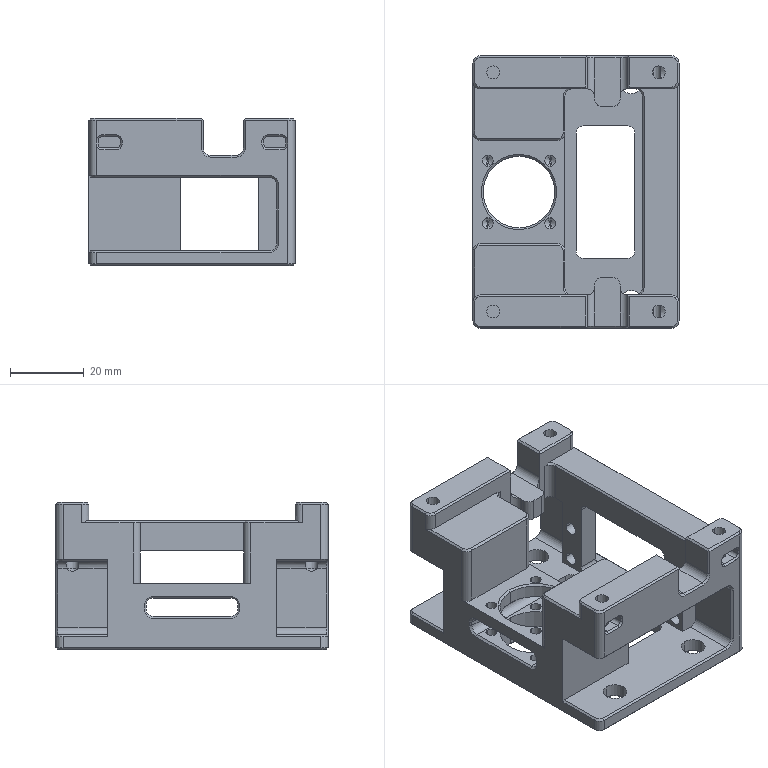NC program | Mastercam | posted with a generic post | part box 56 x 74 x 40 mm
Lines 4683 to 6480 of 45205, first 1525 of 1798 lines:
(3 FEM |TOOL - 3|DIA. OFF. - 3|LEN. - 3|TOOL DIA. - 3.)
N9410 T3 M6
N9412 G0 G54 G90 X10.5 Y9.5 C0. B0. S6000 M3
N9414 G43 H3 Z50.
N9416 Z1.
N9418 G1 Z0. F600.
N9420 X-10.5 Z-.111 F1500.
N9422 G3 X-11. Y9. Z-.116 J-.5
N9424 G1 Y8. Z-.121
N9426 X-10.976 Y7.845 Z-.122
N9428 X-10.905 Y7.706 Z-.123
N9430 X-10.794 Y7.595
N9432 X-10.655 Y7.524 Z-.124
N9434 X-10.5 Y7.5 Z-.125
N9436 X10.5 Z-.236
N9438 G3 X11. Y8. Z-.241 J.5
N9440 G1 Y9. Z-.246
N9442 X10.976 Y9.155 Z-.247
N9444 X10.905 Y9.294 Z-.248
N9446 X10.794 Y9.405
N9448 X10.655 Y9.476 Z-.249
N9450 X10.5 Y9.5 Z-.25
N9452 X-10.5 Z-.361
N9454 G3 X-11. Y9. Z-.366 J-.5
N9456 G1 Y8. Z-.371
N9458 X-10.976 Y7.845 Z-.372
N9460 X-10.905 Y7.706 Z-.373
N9462 X-10.794 Y7.595
N9464 X-10.655 Y7.524 Z-.374
N9466 X-10.5 Y7.5 Z-.375
N9468 X10.5 Z-.486
N9470 G3 X11. Y8. Z-.491 J.5
N9472 G1 Y9. Z-.496
N9474 X10.976 Y9.155 Z-.497
N9476 X10.905 Y9.294 Z-.498
N9478 X10.794 Y9.405
N9480 X10.655 Y9.476 Z-.499
N9482 X10.5 Y9.5 Z-.5
N9484 X-10.5 Z-.611
N9486 G3 X-11. Y9. Z-.616 J-.5
N9488 G1 Y8. Z-.621
N9490 X-10.976 Y7.845 Z-.622
N9492 X-10.905 Y7.706 Z-.623
N9494 X-10.794 Y7.595
N9496 X-10.655 Y7.524 Z-.624
N9498 X-10.5 Y7.5 Z-.625
N9500 X10.5 Z-.736
N9502 G3 X11. Y8. Z-.741 J.5
N9504 G1 Y9. Z-.746
N9506 X10.976 Y9.155 Z-.747
N9508 X10.905 Y9.294 Z-.748
N9510 X10.794 Y9.405
N9512 X10.655 Y9.476 Z-.749
N9514 X10.5 Y9.5 Z-.75
N9516 X-10.5 Z-.861
N9518 G3 X-11. Y9. Z-.866 J-.5
N9520 G1 Y8. Z-.871
N9522 X-10.976 Y7.845 Z-.872
N9524 X-10.905 Y7.706 Z-.873
N9526 X-10.794 Y7.595
N9528 X-10.655 Y7.524 Z-.874
N9530 X-10.5 Y7.5 Z-.875
N9532 X10.5 Z-.986
N9534 G3 X11. Y8. Z-.991 J.5
N9536 G1 Y9. Z-.996
N9538 X10.976 Y9.155 Z-.997
N9540 X10.905 Y9.294 Z-.998
N9542 X10.794 Y9.405
N9544 X10.655 Y9.476 Z-.999
N9546 X10.5 Y9.5 Z-1.
N9548 X-10.5 Z-1.111
N9550 G3 X-11. Y9. Z-1.116 J-.5
N9552 G1 Y8. Z-1.121
N9554 X-10.976 Y7.845 Z-1.122
N9556 X-10.905 Y7.706 Z-1.123
N9558 X-10.794 Y7.595
N9560 X-10.655 Y7.524 Z-1.124
N9562 X-10.5 Y7.5 Z-1.125
N9564 X10.5 Z-1.236
N9566 G3 X11. Y8. Z-1.241 J.5
N9568 G1 Y9. Z-1.246
N9570 X10.976 Y9.155 Z-1.247
N9572 X10.905 Y9.294 Z-1.248
N9574 X10.794 Y9.405
N9576 X10.655 Y9.476 Z-1.249
N9578 X10.5 Y9.5 Z-1.25
N9580 X-10.5 Z-1.361
N9582 G3 X-11. Y9. Z-1.366 J-.5
N9584 G1 Y8. Z-1.371
N9586 X-10.976 Y7.845 Z-1.372
N9588 X-10.905 Y7.706 Z-1.373
N9590 X-10.794 Y7.595
N9592 X-10.655 Y7.524 Z-1.374
N9594 X-10.5 Y7.5 Z-1.375
N9596 X10.5 Z-1.486
N9598 G3 X11. Y8. Z-1.491 J.5
N9600 G1 Y9. Z-1.496
N9602 X10.976 Y9.155 Z-1.497
N9604 X10.905 Y9.294 Z-1.498
N9606 X10.794 Y9.405
N9608 X10.655 Y9.476 Z-1.499
N9610 X10.5 Y9.5 Z-1.5
N9612 X-10.5 Z-1.611
N9614 G3 X-11. Y9. Z-1.616 J-.5
N9616 G1 Y8. Z-1.621
N9618 X-10.976 Y7.845 Z-1.622
N9620 X-10.905 Y7.706 Z-1.623
N9622 X-10.794 Y7.595
N9624 X-10.655 Y7.524 Z-1.624
N9626 X-10.5 Y7.5 Z-1.625
N9628 X10.5 Z-1.736
N9630 G3 X11. Y8. Z-1.741 J.5
N9632 G1 Y9. Z-1.746
N9634 X10.976 Y9.155 Z-1.747
N9636 X10.905 Y9.294 Z-1.748
N9638 X10.794 Y9.405
N9640 X10.655 Y9.476 Z-1.749
N9642 X10.5 Y9.5 Z-1.75
N9644 X-10.5 Z-1.861
N9646 G3 X-11. Y9. Z-1.866 J-.5
N9648 G1 Y8. Z-1.871
N9650 X-10.976 Y7.845 Z-1.872
N9652 X-10.905 Y7.706 Z-1.873
N9654 X-10.794 Y7.595
N9656 X-10.655 Y7.524 Z-1.874
N9658 X-10.5 Y7.5 Z-1.875
N9660 X10.5 Z-1.986
N9662 G3 X11. Y8. Z-1.991 J.5
N9664 G1 Y9. Z-1.996
N9666 X10.976 Y9.155 Z-1.997
N9668 X10.905 Y9.294 Z-1.998
N9670 X10.794 Y9.405
N9672 X10.655 Y9.476 Z-1.999
N9674 X10.5 Y9.5 Z-2.
N9676 X-10.5 Z-2.111
N9678 G3 X-11. Y9. Z-2.116 J-.5
N9680 G1 Y8. Z-2.121
N9682 X-10.976 Y7.845 Z-2.122
N9684 X-10.905 Y7.706 Z-2.123
N9686 X-10.794 Y7.595
N9688 X-10.655 Y7.524 Z-2.124
N9690 X-10.5 Y7.5 Z-2.125
N9692 X10.5 Z-2.236
N9694 G3 X11. Y8. Z-2.241 J.5
N9696 G1 Y9. Z-2.246
N9698 X10.976 Y9.155 Z-2.247
N9700 X10.905 Y9.294 Z-2.248
N9702 X10.794 Y9.405
N9704 X10.655 Y9.476 Z-2.249
N9706 X10.5 Y9.5 Z-2.25
N9708 X-10.5 Z-2.361
N9710 G3 X-11. Y9. Z-2.366 J-.5
N9712 G1 Y8. Z-2.371
N9714 X-10.976 Y7.845 Z-2.372
N9716 X-10.905 Y7.706 Z-2.373
N9718 X-10.794 Y7.595
N9720 X-10.655 Y7.524 Z-2.374
N9722 X-10.5 Y7.5 Z-2.375
N9724 X10.5 Z-2.486
N9726 G3 X11. Y8. Z-2.491 J.5
N9728 G1 Y9. Z-2.496
N9730 X10.976 Y9.155 Z-2.497
N9732 X10.905 Y9.294 Z-2.498
N9734 X10.794 Y9.405
N9736 X10.655 Y9.476 Z-2.499
N9738 X10.5 Y9.5 Z-2.5
N9740 X-10.5 Z-2.611
N9742 G3 X-11. Y9. Z-2.616 J-.5
N9744 G1 Y8. Z-2.621
N9746 X-10.976 Y7.845 Z-2.622
N9748 X-10.905 Y7.706 Z-2.623
N9750 X-10.794 Y7.595
N9752 X-10.655 Y7.524 Z-2.624
N9754 X-10.5 Y7.5 Z-2.625
N9756 X10.5 Z-2.736
N9758 G3 X11. Y8. Z-2.741 J.5
N9760 G1 Y9. Z-2.746
N9762 X10.976 Y9.155 Z-2.747
N9764 X10.905 Y9.294 Z-2.748
N9766 X10.794 Y9.405
N9768 X10.655 Y9.476 Z-2.749
N9770 X10.5 Y9.5 Z-2.75
N9772 X-10.5 Z-2.861
N9774 G3 X-11. Y9. Z-2.866 J-.5
N9776 G1 Y8. Z-2.871
N9778 X-10.976 Y7.845 Z-2.872
N9780 X-10.905 Y7.706 Z-2.873
N9782 X-10.794 Y7.595
N9784 X-10.655 Y7.524 Z-2.874
N9786 X-10.5 Y7.5 Z-2.875
N9788 X10.5 Z-2.986
N9790 G3 X11. Y8. Z-2.991 J.5
N9792 G1 Y9. Z-2.996
N9794 X10.976 Y9.155 Z-2.997
N9796 X10.905 Y9.294 Z-2.998
N9798 X10.794 Y9.405
N9800 X10.655 Y9.476 Z-2.999
N9802 X10.5 Y9.5 Z-3.
N9804 X-10.5 Z-3.111
N9806 G3 X-11. Y9. Z-3.116 J-.5
N9808 G1 Y8. Z-3.121
N9810 X-10.976 Y7.845 Z-3.122
N9812 X-10.905 Y7.706 Z-3.123
N9814 X-10.794 Y7.595
N9816 X-10.655 Y7.524 Z-3.124
N9818 X-10.5 Y7.5 Z-3.125
N9820 X10.5 Z-3.236
N9822 G3 X11. Y8. Z-3.241 J.5
N9824 G1 Y9. Z-3.246
N9826 X10.976 Y9.155 Z-3.247
N9828 X10.905 Y9.294 Z-3.248
N9830 X10.794 Y9.405
N9832 X10.655 Y9.476 Z-3.249
N9834 X10.5 Y9.5 Z-3.25
N9836 X-10.5 Z-3.361
N9838 G3 X-11. Y9. Z-3.366 J-.5
N9840 G1 Y8. Z-3.371
N9842 X-10.976 Y7.845 Z-3.372
N9844 X-10.905 Y7.706 Z-3.373
N9846 X-10.794 Y7.595
N9848 X-10.655 Y7.524 Z-3.374
N9850 X-10.5 Y7.5 Z-3.375
N9852 X10.5 Z-3.486
N9854 G3 X11. Y8. Z-3.491 J.5
N9856 G1 Y9. Z-3.496
N9858 X10.976 Y9.155 Z-3.497
N9860 X10.905 Y9.294 Z-3.498
N9862 X10.794 Y9.405
N9864 X10.655 Y9.476 Z-3.499
N9866 X10.5 Y9.5 Z-3.5
N9868 X-10.5 Z-3.611
N9870 G3 X-11. Y9. Z-3.616 J-.5
N9872 G1 Y8. Z-3.621
N9874 X-10.976 Y7.845 Z-3.622
N9876 X-10.905 Y7.706 Z-3.623
N9878 X-10.794 Y7.595
N9880 X-10.655 Y7.524 Z-3.624
N9882 X-10.5 Y7.5 Z-3.625
N9884 X10.5 Z-3.736
N9886 G3 X11. Y8. Z-3.741 J.5
N9888 G1 Y9. Z-3.746
N9890 X10.976 Y9.155 Z-3.747
N9892 X10.905 Y9.294 Z-3.748
N9894 X10.794 Y9.405
N9896 X10.655 Y9.476 Z-3.749
N9898 X10.5 Y9.5 Z-3.75
N9900 X-10.5 Z-3.861
N9902 G3 X-11. Y9. Z-3.866 J-.5
N9904 G1 Y8. Z-3.871
N9906 X-10.976 Y7.845 Z-3.872
N9908 X-10.905 Y7.706 Z-3.873
N9910 X-10.794 Y7.595
N9912 X-10.655 Y7.524 Z-3.874
N9914 X-10.5 Y7.5 Z-3.875
N9916 X10.5 Z-3.986
N9918 G3 X11. Y8. Z-3.991 J.5
N9920 G1 Y9. Z-3.996
N9922 X10.976 Y9.155 Z-3.997
N9924 X10.905 Y9.294 Z-3.998
N9926 X10.794 Y9.405
N9928 X10.655 Y9.476 Z-3.999
N9930 X10.5 Y9.5 Z-4.
N9932 X-10.5 Z-4.111
N9934 G3 X-11. Y9. Z-4.116 J-.5
N9936 G1 Y8. Z-4.121
N9938 X-10.976 Y7.845 Z-4.122
N9940 X-10.905 Y7.706 Z-4.123
N9942 X-10.794 Y7.595
N9944 X-10.655 Y7.524 Z-4.124
N9946 X-10.5 Y7.5 Z-4.125
N9948 X10.5 Z-4.236
N9950 G3 X11. Y8. Z-4.241 J.5
N9952 G1 Y9. Z-4.246
N9954 X10.976 Y9.155 Z-4.247
N9956 X10.905 Y9.294 Z-4.248
N9958 X10.794 Y9.405
N9960 X10.655 Y9.476 Z-4.249
N9962 X10.5 Y9.5 Z-4.25
N9964 X-10.5 Z-4.361
N9966 G3 X-11. Y9. Z-4.366 J-.5
N9968 G1 Y8. Z-4.371
N9970 X-10.976 Y7.845 Z-4.372
N9972 X-10.905 Y7.706 Z-4.373
N9974 X-10.794 Y7.595
N9976 X-10.655 Y7.524 Z-4.374
N9978 X-10.5 Y7.5 Z-4.375
N9980 X10.5 Z-4.486
N9982 G3 X11. Y8. Z-4.491 J.5
N9984 G1 Y9. Z-4.496
N9986 X10.976 Y9.155 Z-4.497
N9988 X10.905 Y9.294 Z-4.498
N9990 X10.794 Y9.405
N9992 X10.655 Y9.476 Z-4.499
N9994 X10.5 Y9.5 Z-4.5
N9996 X-10.5 Z-4.611
N9998 G3 X-11. Y9. Z-4.616 J-.5
N100 G1 Y8. Z-4.621
N102 X-10.976 Y7.845 Z-4.622
N104 X-10.905 Y7.706 Z-4.623
N106 X-10.794 Y7.595
N108 X-10.655 Y7.524 Z-4.624
N110 X-10.5 Y7.5 Z-4.625
N112 X10.5 Z-4.736
N114 G3 X11. Y8. Z-4.741 J.5
N116 G1 Y9. Z-4.746
N118 X10.976 Y9.155 Z-4.747
N120 X10.905 Y9.294 Z-4.748
N122 X10.794 Y9.405
N124 X10.655 Y9.476 Z-4.749
N126 X10.5 Y9.5 Z-4.75
N128 X-10.5 Z-4.861
N130 G3 X-11. Y9. Z-4.866 J-.5
N132 G1 Y8. Z-4.871
N134 X-10.976 Y7.845 Z-4.872
N136 X-10.905 Y7.706 Z-4.873
N138 X-10.794 Y7.595
N140 X-10.655 Y7.524 Z-4.874
N142 X-10.5 Y7.5 Z-4.875
N144 X10.5 Z-4.986
N146 G3 X11. Y8. Z-4.991 J.5
N148 G1 Y9. Z-4.996
N150 X10.976 Y9.155 Z-4.997
N152 X10.905 Y9.294 Z-4.998
N154 X10.794 Y9.405
N156 X10.655 Y9.476 Z-4.999
N158 X10.5 Y9.5 Z-5.
N160 X-10.5 Z-5.111
N162 G3 X-11. Y9. Z-5.116 J-.5
N164 G1 Y8. Z-5.121
N166 X-10.976 Y7.845 Z-5.122
N168 X-10.905 Y7.706 Z-5.123
N170 X-10.794 Y7.595
N172 X-10.655 Y7.524 Z-5.124
N174 X-10.5 Y7.5 Z-5.125
N176 X10.5 Z-5.236
N178 G3 X11. Y8. Z-5.241 J.5
N180 G1 Y9. Z-5.246
N182 X10.976 Y9.155 Z-5.247
N184 X10.905 Y9.294 Z-5.248
N186 X10.794 Y9.405
N188 X10.655 Y9.476 Z-5.249
N190 X10.5 Y9.5 Z-5.25
N192 X-10.5 Z-5.361
N194 G3 X-11. Y9. Z-5.366 J-.5
N196 G1 Y8. Z-5.371
N198 X-10.976 Y7.845 Z-5.372
N200 X-10.905 Y7.706 Z-5.373
N202 X-10.794 Y7.595
N204 X-10.655 Y7.524 Z-5.374
N206 X-10.5 Y7.5 Z-5.375
N208 X10.5 Z-5.486
N210 G3 X11. Y8. Z-5.491 J.5
N212 G1 Y9. Z-5.496
N214 X10.976 Y9.155 Z-5.497
N216 X10.905 Y9.294 Z-5.498
N218 X10.794 Y9.405
N220 X10.655 Y9.476 Z-5.499
N222 X10.5 Y9.5 Z-5.5
N224 X-10.5 Z-5.611
N226 G3 X-11. Y9. Z-5.616 J-.5
N228 G1 Y8. Z-5.621
N230 X-10.976 Y7.845 Z-5.622
N232 X-10.905 Y7.706 Z-5.623
N234 X-10.794 Y7.595
N236 X-10.655 Y7.524 Z-5.624
N238 X-10.5 Y7.5 Z-5.625
N240 X10.5 Z-5.736
N242 G3 X11. Y8. Z-5.741 J.5
N244 G1 Y9. Z-5.746
N246 X10.976 Y9.155 Z-5.747
N248 X10.905 Y9.294 Z-5.748
N250 X10.794 Y9.405
N252 X10.655 Y9.476 Z-5.749
N254 X10.5 Y9.5 Z-5.75
N256 X-10.5 Z-5.861
N258 G3 X-11. Y9. Z-5.866 J-.5
N260 G1 Y8. Z-5.871
N262 X-10.976 Y7.845 Z-5.872
N264 X-10.905 Y7.706 Z-5.873
N266 X-10.794 Y7.595
N268 X-10.655 Y7.524 Z-5.874
N270 X-10.5 Y7.5 Z-5.875
N272 X10.5 Z-5.986
N274 G3 X11. Y8. Z-5.991 J.5
N276 G1 Y9. Z-5.996
N278 X10.976 Y9.155 Z-5.997
N280 X10.905 Y9.294 Z-5.998
N282 X10.794 Y9.405
N284 X10.655 Y9.476 Z-5.999
N286 X10.5 Y9.5 Z-6.
N288 X-10.5 Z-6.111
N290 G3 X-11. Y9. Z-6.116 J-.5
N292 G1 Y8. Z-6.121
N294 X-10.976 Y7.845 Z-6.122
N296 X-10.905 Y7.706 Z-6.123
N298 X-10.794 Y7.595
N300 X-10.655 Y7.524 Z-6.124
N302 X-10.5 Y7.5 Z-6.125
N304 X10.5 Z-6.236
N306 G3 X11. Y8. Z-6.241 J.5
N308 G1 Y9. Z-6.246
N310 X10.976 Y9.155 Z-6.247
N312 X10.905 Y9.294 Z-6.248
N314 X10.794 Y9.405
N316 X10.655 Y9.476 Z-6.249
N318 X10.5 Y9.5 Z-6.25
N320 X-10.5 Z-6.361
N322 G3 X-11. Y9. Z-6.366 J-.5
N324 G1 Y8. Z-6.371
N326 X-10.976 Y7.845 Z-6.372
N328 X-10.905 Y7.706 Z-6.373
N330 X-10.794 Y7.595
N332 X-10.655 Y7.524 Z-6.374
N334 X-10.5 Y7.5 Z-6.375
N336 X10.5 Z-6.486
N338 G3 X11. Y8. Z-6.491 J.5
N340 G1 Y9. Z-6.496
N342 X10.976 Y9.155 Z-6.497
N344 X10.905 Y9.294 Z-6.498
N346 X10.794 Y9.405
N348 X10.655 Y9.476 Z-6.499
N350 X10.5 Y9.5 Z-6.5
N352 X-10.5 Z-6.611
N354 G3 X-11. Y9. Z-6.616 J-.5
N356 G1 Y8. Z-6.621
N358 X-10.976 Y7.845 Z-6.622
N360 X-10.905 Y7.706 Z-6.623
N362 X-10.794 Y7.595
N364 X-10.655 Y7.524 Z-6.624
N366 X-10.5 Y7.5 Z-6.625
N368 X10.5 Z-6.736
N370 G3 X11. Y8. Z-6.741 J.5
N372 G1 Y9. Z-6.746
N374 X10.976 Y9.155 Z-6.747
N376 X10.905 Y9.294 Z-6.748
N378 X10.794 Y9.405
N380 X10.655 Y9.476 Z-6.749
N382 X10.5 Y9.5 Z-6.75
N384 X-10.5 Z-6.861
N386 G3 X-11. Y9. Z-6.866 J-.5
N388 G1 Y8. Z-6.871
N390 X-10.976 Y7.845 Z-6.872
N392 X-10.905 Y7.706 Z-6.873
N394 X-10.794 Y7.595
N396 X-10.655 Y7.524 Z-6.874
N398 X-10.5 Y7.5 Z-6.875
N400 X10.5 Z-6.986
N402 G3 X11. Y8. Z-6.991 J.5
N404 G1 Y9. Z-6.996
N406 X10.976 Y9.155 Z-6.997
N408 X10.905 Y9.294 Z-6.998
N410 X10.794 Y9.405
N412 X10.655 Y9.476 Z-6.999
N414 X10.5 Y9.5 Z-7.
N416 X-10.5 Z-7.111
N418 G3 X-11. Y9. Z-7.116 J-.5
N420 G1 Y8. Z-7.121
N422 X-10.976 Y7.845 Z-7.122
N424 X-10.905 Y7.706 Z-7.123
N426 X-10.794 Y7.595
N428 X-10.655 Y7.524 Z-7.124
N430 X-10.5 Y7.5 Z-7.125
N432 X10.5 Z-7.236
N434 G3 X11. Y8. Z-7.241 J.5
N436 G1 Y9. Z-7.246
N438 X10.976 Y9.155 Z-7.247
N440 X10.905 Y9.294 Z-7.248
N442 X10.794 Y9.405
N444 X10.655 Y9.476 Z-7.249
N446 X10.5 Y9.5 Z-7.25
N448 X-10.5 Z-7.361
N450 G3 X-11. Y9. Z-7.366 J-.5
N452 G1 Y8. Z-7.371
N454 X-10.976 Y7.845 Z-7.372
N456 X-10.905 Y7.706 Z-7.373
N458 X-10.794 Y7.595
N460 X-10.655 Y7.524 Z-7.374
N462 X-10.5 Y7.5 Z-7.375
N464 X10.5 Z-7.486
N466 G3 X11. Y8. Z-7.491 J.5
N468 G1 Y9. Z-7.496
N470 X10.976 Y9.155 Z-7.497
N472 X10.905 Y9.294 Z-7.498
N474 X10.794 Y9.405
N476 X10.655 Y9.476 Z-7.499
N478 X10.5 Y9.5 Z-7.5
N480 X-10.5 Z-7.611
N482 G3 X-11. Y9. Z-7.616 J-.5
N484 G1 Y8. Z-7.621
N486 X-10.976 Y7.845 Z-7.622
N488 X-10.905 Y7.706 Z-7.623
N490 X-10.794 Y7.595
N492 X-10.655 Y7.524 Z-7.624
N494 X-10.5 Y7.5 Z-7.625
N496 X10.5 Z-7.736
N498 G3 X11. Y8. Z-7.741 J.5
N500 G1 Y9. Z-7.746
N502 X10.976 Y9.155 Z-7.747
N504 X10.905 Y9.294 Z-7.748
N506 X10.794 Y9.405
N508 X10.655 Y9.476 Z-7.749
N510 X10.5 Y9.5 Z-7.75
N512 X-10.5 Z-7.861
N514 G3 X-11. Y9. Z-7.866 J-.5
N516 G1 Y8. Z-7.871
N518 X-10.976 Y7.845 Z-7.872
N520 X-10.905 Y7.706 Z-7.873
N522 X-10.794 Y7.595
N524 X-10.655 Y7.524 Z-7.874
N526 X-10.5 Y7.5 Z-7.875
N528 X10.5 Z-7.986
N530 G3 X11. Y8. Z-7.991 J.5
N532 G1 Y9. Z-7.996
N534 X10.976 Y9.155 Z-7.997
N536 X10.905 Y9.294 Z-7.998
N538 X10.794 Y9.405
N540 X10.655 Y9.476 Z-7.999
N542 X10.5 Y9.5 Z-8.
N544 X-10.5 Z-8.111
N546 G3 X-11. Y9. Z-8.116 J-.5
N548 G1 Y8. Z-8.121
N550 X-10.976 Y7.845 Z-8.122
N552 X-10.905 Y7.706 Z-8.123
N554 X-10.794 Y7.595
N556 X-10.655 Y7.524 Z-8.124
N558 X-10.5 Y7.5 Z-8.125
N560 X10.5 Z-8.236
N562 G3 X11. Y8. Z-8.241 J.5
N564 G1 Y9. Z-8.246
N566 X10.976 Y9.155 Z-8.247
N568 X10.905 Y9.294 Z-8.248
N570 X10.794 Y9.405
N572 X10.655 Y9.476 Z-8.249
N574 X10.5 Y9.5 Z-8.25
N576 X-10.5 Z-8.361
N578 G3 X-11. Y9. Z-8.366 J-.5
N580 G1 Y8. Z-8.371
N582 X-10.976 Y7.845 Z-8.372
N584 X-10.905 Y7.706 Z-8.373
N586 X-10.794 Y7.595
N588 X-10.655 Y7.524 Z-8.374
N590 X-10.5 Y7.5 Z-8.375
N592 X10.5 Z-8.486
N594 G3 X11. Y8. Z-8.491 J.5
N596 G1 Y9. Z-8.496
N598 X10.976 Y9.155 Z-8.497
N600 X10.905 Y9.294 Z-8.498
N602 X10.794 Y9.405
N604 X10.655 Y9.476 Z-8.499
N606 X10.5 Y9.5 Z-8.5
N608 X-10.5 Z-8.611
N610 G3 X-11. Y9. Z-8.616 J-.5
N612 G1 Y8. Z-8.621
N614 X-10.976 Y7.845 Z-8.622
N616 X-10.905 Y7.706 Z-8.623
N618 X-10.794 Y7.595
N620 X-10.655 Y7.524 Z-8.624
N622 X-10.5 Y7.5 Z-8.625
N624 X10.5 Z-8.736
N626 G3 X11. Y8. Z-8.741 J.5
N628 G1 Y9. Z-8.746
N630 X10.976 Y9.155 Z-8.747
N632 X10.905 Y9.294 Z-8.748
N634 X10.794 Y9.405
N636 X10.655 Y9.476 Z-8.749
N638 X10.5 Y9.5 Z-8.75
N640 X-10.5 Z-8.861
N642 G3 X-11. Y9. Z-8.866 J-.5
N644 G1 Y8. Z-8.871
N646 X-10.976 Y7.845 Z-8.872
N648 X-10.905 Y7.706 Z-8.873
N650 X-10.794 Y7.595
N652 X-10.655 Y7.524 Z-8.874
N654 X-10.5 Y7.5 Z-8.875
N656 X10.5 Z-8.986
N658 G3 X11. Y8. Z-8.991 J.5
N660 G1 Y9. Z-8.996
N662 X10.976 Y9.155 Z-8.997
N664 X10.905 Y9.294 Z-8.998
N666 X10.794 Y9.405
N668 X10.655 Y9.476 Z-8.999
N670 X10.5 Y9.5 Z-9.
N672 X-10.5 Z-9.111
N674 G3 X-11. Y9. Z-9.116 J-.5
N676 G1 Y8. Z-9.121
N678 X-10.976 Y7.845 Z-9.122
N680 X-10.905 Y7.706 Z-9.123
N682 X-10.794 Y7.595
N684 X-10.655 Y7.524 Z-9.124
N686 X-10.5 Y7.5 Z-9.125
N688 X10.5 Z-9.236
N690 G3 X11. Y8. Z-9.241 J.5
N692 G1 Y9. Z-9.246
N694 X10.976 Y9.155 Z-9.247
N696 X10.905 Y9.294 Z-9.248
N698 X10.794 Y9.405
N700 X10.655 Y9.476 Z-9.249
N702 X10.5 Y9.5 Z-9.25
N704 X-10.5 Z-9.361
N706 G3 X-11. Y9. Z-9.366 J-.5
N708 G1 Y8. Z-9.371
N710 X-10.976 Y7.845 Z-9.372
N712 X-10.905 Y7.706 Z-9.373
N714 X-10.794 Y7.595
N716 X-10.655 Y7.524 Z-9.374
N718 X-10.5 Y7.5 Z-9.375
N720 X10.5 Z-9.486
N722 G3 X11. Y8. Z-9.491 J.5
N724 G1 Y9. Z-9.496
N726 X10.976 Y9.155 Z-9.497
N728 X10.905 Y9.294 Z-9.498
N730 X10.794 Y9.405
N732 X10.655 Y9.476 Z-9.499
N734 X10.5 Y9.5 Z-9.5
N736 X-10.5 Z-9.611
N738 G3 X-11. Y9. Z-9.616 J-.5
N740 G1 Y8. Z-9.621
N742 X-10.976 Y7.845 Z-9.622
N744 X-10.905 Y7.706 Z-9.623
N746 X-10.794 Y7.595
N748 X-10.655 Y7.524 Z-9.624
N750 X-10.5 Y7.5 Z-9.625
N752 X10.5 Z-9.736
N754 G3 X11. Y8. Z-9.741 J.5
N756 G1 Y9. Z-9.746
N758 X10.976 Y9.155 Z-9.747
N760 X10.905 Y9.294 Z-9.748
N762 X10.794 Y9.405
N764 X10.655 Y9.476 Z-9.749
N766 X10.5 Y9.5 Z-9.75
N768 X-10.5 Z-9.861
N770 G3 X-11. Y9. Z-9.866 J-.5
N772 G1 Y8. Z-9.871
N774 X-10.976 Y7.845 Z-9.872
N776 X-10.905 Y7.706 Z-9.873
N778 X-10.794 Y7.595
N780 X-10.655 Y7.524 Z-9.874
N782 X-10.5 Y7.5 Z-9.875
N784 X10.5 Z-9.986
N786 G3 X11. Y8. Z-9.991 J.5
N788 G1 Y9. Z-9.996
N790 X10.976 Y9.155 Z-9.997
N792 X10.905 Y9.294 Z-9.998
N794 X10.794 Y9.405
N796 X10.655 Y9.476 Z-9.999
N798 X10.5 Y9.5 Z-10.
N800 X-10.5 Z-10.111
N802 G3 X-11. Y9. Z-10.116 J-.5
N804 G1 Y8. Z-10.121
N806 X-10.976 Y7.845 Z-10.122
N808 X-10.905 Y7.706 Z-10.123
N810 X-10.794 Y7.595
N812 X-10.655 Y7.524 Z-10.124
N814 X-10.5 Y7.5 Z-10.125
N816 X10.5 Z-10.236
N818 G3 X11. Y8. Z-10.241 J.5
N820 G1 Y9. Z-10.246
N822 X10.976 Y9.155 Z-10.247
N824 X10.905 Y9.294 Z-10.248
N826 X10.794 Y9.405
N828 X10.655 Y9.476 Z-10.249
N830 X10.5 Y9.5 Z-10.25
N832 X-10.5 Z-10.361
N834 G3 X-11. Y9. Z-10.366 J-.5
N836 G1 Y8. Z-10.371
N838 X-10.976 Y7.845 Z-10.372
N840 X-10.905 Y7.706 Z-10.373
N842 X-10.794 Y7.595
N844 X-10.655 Y7.524 Z-10.374
N846 X-10.5 Y7.5 Z-10.375
N848 X10.5 Z-10.486
N850 G3 X11. Y8. Z-10.491 J.5
N852 G1 Y9. Z-10.496
N854 X10.976 Y9.155 Z-10.497
N856 X10.905 Y9.294 Z-10.498
N858 X10.794 Y9.405
N860 X10.655 Y9.476 Z-10.499
N862 X10.5 Y9.5 Z-10.5
N864 X-10.5 Z-10.611
N866 G3 X-11. Y9. Z-10.616 J-.5
N868 G1 Y8. Z-10.621
N870 X-10.976 Y7.845 Z-10.622
N872 X-10.905 Y7.706 Z-10.623
N874 X-10.794 Y7.595
N876 X-10.655 Y7.524 Z-10.624
N878 X-10.5 Y7.5 Z-10.625
N880 X10.5 Z-10.736
N882 G3 X11. Y8. Z-10.741 J.5
N884 G1 Y9. Z-10.746
N886 X10.976 Y9.155 Z-10.747
N888 X10.905 Y9.294 Z-10.748
N890 X10.794 Y9.405
N892 X10.655 Y9.476 Z-10.749
N894 X10.5 Y9.5 Z-10.75
N896 X-10.5 Z-10.861
N898 G3 X-11. Y9. Z-10.866 J-.5
N900 G1 Y8. Z-10.871
N902 X-10.976 Y7.845 Z-10.872
N904 X-10.905 Y7.706 Z-10.873
N906 X-10.794 Y7.595
N908 X-10.655 Y7.524 Z-10.874
N910 X-10.5 Y7.5 Z-10.875
N912 X10.5 Z-10.986
N914 G3 X11. Y8. Z-10.991 J.5
N916 G1 Y9. Z-10.996
N918 X10.976 Y9.155 Z-10.997
N920 X10.905 Y9.294 Z-10.998
N922 X10.794 Y9.405
N924 X10.655 Y9.476 Z-10.999
N926 X10.5 Y9.5 Z-11.
N928 X-10.5 Z-11.111
N930 G3 X-11. Y9. Z-11.116 J-.5
N932 G1 Y8. Z-11.121
N934 X-10.976 Y7.845 Z-11.122
N936 X-10.905 Y7.706 Z-11.123
N938 X-10.794 Y7.595
N940 X-10.655 Y7.524 Z-11.124
N942 X-10.5 Y7.5 Z-11.125
N944 X10.5 Z-11.236
N946 G3 X11. Y8. Z-11.241 J.5
N948 G1 Y9. Z-11.246
N950 X10.976 Y9.155 Z-11.247
N952 X10.905 Y9.294 Z-11.248
N954 X10.794 Y9.405
N956 X10.655 Y9.476 Z-11.249
N958 X10.5 Y9.5 Z-11.25
N960 X-10.5 Z-11.361
N962 G3 X-11. Y9. Z-11.366 J-.5
N964 G1 Y8. Z-11.371
N966 X-10.976 Y7.845 Z-11.372
N968 X-10.905 Y7.706 Z-11.373
N970 X-10.794 Y7.595
N972 X-10.655 Y7.524 Z-11.374
N974 X-10.5 Y7.5 Z-11.375
N976 X10.5 Z-11.486
N978 G3 X11. Y8. Z-11.491 J.5
N980 G1 Y9. Z-11.496
N982 X10.976 Y9.155 Z-11.497
N984 X10.905 Y9.294 Z-11.498
N986 X10.794 Y9.405
N988 X10.655 Y9.476 Z-11.499
N990 X10.5 Y9.5 Z-11.5
N992 X-10.5 Z-11.611
N994 G3 X-11. Y9. Z-11.616 J-.5
N996 G1 Y8. Z-11.621
N998 X-10.976 Y7.845 Z-11.622
N1000 X-10.905 Y7.706 Z-11.623
N1002 X-10.794 Y7.595
N1004 X-10.655 Y7.524 Z-11.624
N1006 X-10.5 Y7.5 Z-11.625
N1008 X10.5 Z-11.736
N1010 G3 X11. Y8. Z-11.741 J.5
N1012 G1 Y9. Z-11.746
N1014 X10.976 Y9.155 Z-11.747
N1016 X10.905 Y9.294 Z-11.748
N1018 X10.794 Y9.405
N1020 X10.655 Y9.476 Z-11.749
N1022 X10.5 Y9.5 Z-11.75
N1024 X-10.5 Z-11.861
N1026 G3 X-11. Y9. Z-11.866 J-.5
N1028 G1 Y8. Z-11.871
N1030 X-10.976 Y7.845 Z-11.872
N1032 X-10.905 Y7.706 Z-11.873
N1034 X-10.794 Y7.595
N1036 X-10.655 Y7.524 Z-11.874
N1038 X-10.5 Y7.5 Z-11.875
N1040 X10.5 Z-11.986
N1042 G3 X11. Y8. Z-11.991 J.5
N1044 G1 Y9. Z-11.996
N1046 X10.976 Y9.155 Z-11.997
N1048 X10.905 Y9.294 Z-11.998
N1050 X10.794 Y9.405
N1052 X10.655 Y9.476 Z-11.999
N1054 X10.5 Y9.5 Z-12.
N1056 X-10.5 Z-12.111
N1058 G3 X-11. Y9. Z-12.116 J-.5
N1060 G1 Y8. Z-12.121
N1062 X-10.976 Y7.845 Z-12.122
N1064 X-10.905 Y7.706 Z-12.123
N1066 X-10.794 Y7.595
N1068 X-10.655 Y7.524 Z-12.124
N1070 X-10.5 Y7.5 Z-12.125
N1072 X10.5 Z-12.236
N1074 G3 X11. Y8. Z-12.241 J.5
N1076 G1 Y9. Z-12.246
N1078 X10.976 Y9.155 Z-12.247
N1080 X10.905 Y9.294 Z-12.248
N1082 X10.794 Y9.405
N1084 X10.655 Y9.476 Z-12.249
N1086 X10.5 Y9.5 Z-12.25
N1088 X-10.5 Z-12.361
N1090 G3 X-11. Y9. Z-12.366 J-.5
N1092 G1 Y8. Z-12.371
N1094 X-10.976 Y7.845 Z-12.372
N1096 X-10.905 Y7.706 Z-12.373
N1098 X-10.794 Y7.595
N1100 X-10.655 Y7.524 Z-12.374
N1102 X-10.5 Y7.5 Z-12.375
N1104 X10.5 Z-12.486
N1106 G3 X11. Y8. Z-12.491 J.5
N1108 G1 Y9. Z-12.496
N1110 X10.976 Y9.155 Z-12.497
N1112 X10.905 Y9.294 Z-12.498
N1114 X10.794 Y9.405
N1116 X10.655 Y9.476 Z-12.499
N1118 X10.5 Y9.5 Z-12.5
N1120 X-10.5 Z-12.611
N1122 G3 X-11. Y9. Z-12.616 J-.5
N1124 G1 Y8. Z-12.621
N1126 X-10.976 Y7.845 Z-12.622
N1128 X-10.905 Y7.706 Z-12.623
N1130 X-10.794 Y7.595
N1132 X-10.655 Y7.524 Z-12.624
N1134 X-10.5 Y7.5 Z-12.625
N1136 X10.5 Z-12.736
N1138 G3 X11. Y8. Z-12.741 J.5
N1140 G1 Y9. Z-12.746
N1142 X10.976 Y9.155 Z-12.747
N1144 X10.905 Y9.294 Z-12.748
N1146 X10.794 Y9.405
N1148 X10.655 Y9.476 Z-12.749
N1150 X10.5 Y9.5 Z-12.75
N1152 X-10.5 Z-12.861
N1154 G3 X-11. Y9. Z-12.866 J-.5
N1156 G1 Y8. Z-12.871
N1158 X-10.976 Y7.845 Z-12.872
N1160 X-10.905 Y7.706 Z-12.873
N1162 X-10.794 Y7.595
N1164 X-10.655 Y7.524 Z-12.874
N1166 X-10.5 Y7.5 Z-12.875
N1168 X10.5 Z-12.986
N1170 G3 X11. Y8. Z-12.991 J.5
N1172 G1 Y9. Z-12.996
N1174 X10.976 Y9.155 Z-12.997
N1176 X10.905 Y9.294 Z-12.998
N1178 X10.794 Y9.405
N1180 X10.655 Y9.476 Z-12.999
N1182 X10.5 Y9.5 Z-13.
N1184 X-10.5 Z-13.111
N1186 G3 X-11. Y9. Z-13.116 J-.5
N1188 G1 Y8. Z-13.121
N1190 X-10.976 Y7.845 Z-13.122
N1192 X-10.905 Y7.706 Z-13.123
N1194 X-10.794 Y7.595
N1196 X-10.655 Y7.524 Z-13.124
N1198 X-10.5 Y7.5 Z-13.125
N1200 X10.5 Z-13.236
N1202 G3 X11. Y8. Z-13.241 J.5
N1204 G1 Y9. Z-13.246
N1206 X10.976 Y9.155 Z-13.247
N1208 X10.905 Y9.294 Z-13.248
N1210 X10.794 Y9.405
N1212 X10.655 Y9.476 Z-13.249
N1214 X10.5 Y9.5 Z-13.25
N1216 X-10.5 Z-13.361
N1218 G3 X-11. Y9. Z-13.366 J-.5
N1220 G1 Y8. Z-13.371
N1222 X-10.976 Y7.845 Z-13.372
N1224 X-10.905 Y7.706 Z-13.373
N1226 X-10.794 Y7.595
N1228 X-10.655 Y7.524 Z-13.374
N1230 X-10.5 Y7.5 Z-13.375
N1232 X10.5 Z-13.486
N1234 G3 X11. Y8. Z-13.491 J.5
N1236 G1 Y9. Z-13.496
N1238 X10.976 Y9.155 Z-13.497
N1240 X10.905 Y9.294 Z-13.498
N1242 X10.794 Y9.405
N1244 X10.655 Y9.476 Z-13.499
N1246 X10.5 Y9.5 Z-13.5
N1248 X-10.5 Z-13.611
N1250 G3 X-11. Y9. Z-13.616 J-.5
N1252 G1 Y8. Z-13.621
N1254 X-10.976 Y7.845 Z-13.622
N1256 X-10.905 Y7.706 Z-13.623
N1258 X-10.794 Y7.595
N1260 X-10.655 Y7.524 Z-13.624
N1262 X-10.5 Y7.5 Z-13.625
N1264 X10.5 Z-13.736
N1266 G3 X11. Y8. Z-13.741 J.5
N1268 G1 Y9. Z-13.746
N1270 X10.976 Y9.155 Z-13.747
N1272 X10.905 Y9.294 Z-13.748
N1274 X10.794 Y9.405
N1276 X10.655 Y9.476 Z-13.749
N1278 X10.5 Y9.5 Z-13.75
N1280 X-10.5 Z-13.861
N1282 G3 X-11. Y9. Z-13.866 J-.5
N1284 G1 Y8. Z-13.871
N1286 X-10.976 Y7.845 Z-13.872
N1288 X-10.905 Y7.706 Z-13.873
N1290 X-10.794 Y7.595
N1292 X-10.655 Y7.524 Z-13.874
N1294 X-10.5 Y7.5 Z-13.875
N1296 X10.5 Z-13.986
N1298 G3 X11. Y8. Z-13.991 J.5
N1300 G1 Y9. Z-13.996
N1302 X10.976 Y9.155 Z-13.997
N1304 X10.905 Y9.294 Z-13.998
N1306 X10.794 Y9.405
N1308 X10.655 Y9.476 Z-13.999
N1310 X10.5 Y9.5 Z-14.
N1312 X-10.5 Z-14.111
N1314 G3 X-11. Y9. Z-14.116 J-.5
N1316 G1 Y8. Z-14.121
N1318 X-10.976 Y7.845 Z-14.122
N1320 X-10.905 Y7.706 Z-14.123
N1322 X-10.794 Y7.595
N1324 X-10.655 Y7.524 Z-14.124
N1326 X-10.5 Y7.5 Z-14.125
N1328 X10.5 Z-14.236
N1330 G3 X11. Y8. Z-14.241 J.5
N1332 G1 Y9. Z-14.246
N1334 X10.976 Y9.155 Z-14.247
N1336 X10.905 Y9.294 Z-14.248
N1338 X10.794 Y9.405
N1340 X10.655 Y9.476 Z-14.249
N1342 X10.5 Y9.5 Z-14.25
N1344 X-10.5 Z-14.361
N1346 G3 X-11. Y9. Z-14.366 J-.5
N1348 G1 Y8. Z-14.371
N1350 X-10.976 Y7.845 Z-14.372
N1352 X-10.905 Y7.706 Z-14.373
N1354 X-10.794 Y7.595
N1356 X-10.655 Y7.524 Z-14.374
N1358 X-10.5 Y7.5 Z-14.375
N1360 X10.5 Z-14.486
N1362 G3 X11. Y8. Z-14.491 J.5
N1364 G1 Y9. Z-14.496
N1366 X10.976 Y9.155 Z-14.497
N1368 X10.905 Y9.294 Z-14.498
N1370 X10.794 Y9.405
N1372 X10.655 Y9.476 Z-14.499
N1374 X10.5 Y9.5 Z-14.5
N1376 X-10.5 Z-14.611
N1378 G3 X-11. Y9. Z-14.616 J-.5
N1380 G1 Y8. Z-14.621
N1382 X-10.976 Y7.845 Z-14.622
N1384 X-10.905 Y7.706 Z-14.623
N1386 X-10.794 Y7.595
N1388 X-10.655 Y7.524 Z-14.624
N1390 X-10.5 Y7.5 Z-14.625
N1392 X10.5 Z-14.736
N1394 G3 X11. Y8. Z-14.741 J.5
N1396 G1 Y9. Z-14.746
N1398 X10.976 Y9.155 Z-14.747
N1400 X10.905 Y9.294 Z-14.748
N1402 X10.794 Y9.405
N1404 X10.655 Y9.476 Z-14.749
N1406 X10.5 Y9.5 Z-14.75
N1408 X-10.5 Z-14.861
N1410 G3 X-11. Y9. Z-14.866 J-.5
N1412 G1 Y8. Z-14.871
N1414 X-10.976 Y7.845 Z-14.872
N1416 X-10.905 Y7.706 Z-14.873
N1418 X-10.794 Y7.595
N1420 X-10.655 Y7.524 Z-14.874
N1422 X-10.5 Y7.5 Z-14.875
N1424 X10.5 Z-14.986
N1426 G3 X11. Y8. Z-14.991 J.5
N1428 G1 Y9. Z-14.996
N1430 X10.976 Y9.155 Z-14.997
N1432 X10.905 Y9.294 Z-14.998
N1434 X10.794 Y9.405
N1436 X10.655 Y9.476 Z-14.999
N1438 X10.5 Y9.5 Z-15.
N1440 X-10.5 Z-15.111
N1442 G3 X-11. Y9. Z-15.116 J-.5
N1444 G1 Y8. Z-15.121
N1446 X-10.976 Y7.845 Z-15.122
N1448 X-10.905 Y7.706 Z-15.123
N1450 X-10.794 Y7.595
N1452 X-10.655 Y7.524 Z-15.124
N1454 X-10.5 Y7.5 Z-15.125
N1456 X10.5 Z-15.236
N1458 G3 X11. Y8. Z-15.241 J.5
N1460 G1 Y9. Z-15.246
N1462 X10.976 Y9.155 Z-15.247
N1464 X10.905 Y9.294 Z-15.248
N1466 X10.794 Y9.405
N1468 X10.655 Y9.476 Z-15.249
N1470 X10.5 Y9.5 Z-15.25
N1472 X-10.5 Z-15.361
N1474 G3 X-11. Y9. Z-15.366 J-.5
N1476 G1 Y8. Z-15.371
N1478 X-10.976 Y7.845 Z-15.372
N1480 X-10.905 Y7.706 Z-15.373
N1482 X-10.794 Y7.595
N1484 X-10.655 Y7.524 Z-15.374
N1486 X-10.5 Y7.5 Z-15.375
N1488 X10.5 Z-15.486
N1490 G3 X11. Y8. Z-15.491 J.5
N1492 G1 Y9. Z-15.496
N1494 X10.976 Y9.155 Z-15.497
N1496 X10.905 Y9.294 Z-15.498
N1498 X10.794 Y9.405
N1500 X10.655 Y9.476 Z-15.499
N1502 X10.5 Y9.5 Z-15.5
N1504 X-10.5 Z-15.611
N1506 G3 X-11. Y9. Z-15.616 J-.5
N1508 G1 Y8. Z-15.621
N1510 X-10.976 Y7.845 Z-15.622
N1512 X-10.905 Y7.706 Z-15.623
N1514 X-10.794 Y7.595
N1516 X-10.655 Y7.524 Z-15.624
N1518 X-10.5 Y7.5 Z-15.625
N1520 X10.5 Z-15.736
N1522 G3 X11. Y8. Z-15.741 J.5
N1524 G1 Y9. Z-15.746
N1526 X10.976 Y9.155 Z-15.747
N1528 X10.905 Y9.294 Z-15.748
N1530 X10.794 Y9.405
N1532 X10.655 Y9.476 Z-15.749
N1534 X10.5 Y9.5 Z-15.75
N1536 X-10.5 Z-15.861
N1538 G3 X-11. Y9. Z-15.866 J-.5
N1540 G1 Y8. Z-15.871
N1542 X-10.976 Y7.845 Z-15.872
N1544 X-10.905 Y7.706 Z-15.873
N1546 X-10.794 Y7.595
N1548 X-10.655 Y7.524 Z-15.874
N1550 X-10.5 Y7.5 Z-15.875
N1552 X10.5 Z-15.986
N1554 G3 X11. Y8. Z-15.991 J.5
N1556 G1 Y9. Z-15.996
N1558 X10.976 Y9.155 Z-15.997
N1560 X10.905 Y9.294 Z-15.998
N1562 X10.794 Y9.405
N1564 X10.655 Y9.476 Z-15.999
N1566 X10.5 Y9.5 Z-16.
N1568 X-10.5 Z-16.111
N1570 G3 X-11. Y9. Z-16.116 J-.5
N1572 G1 Y8. Z-16.121
N1574 X-10.976 Y7.845 Z-16.122
N1576 X-10.905 Y7.706 Z-16.123
N1578 X-10.794 Y7.595
N1580 X-10.655 Y7.524 Z-16.124
N1582 X-10.5 Y7.5 Z-16.125
N1584 X10.5 Z-16.236
N1586 G3 X11. Y8. Z-16.241 J.5
N1588 G1 Y9. Z-16.246
N1590 X10.976 Y9.155 Z-16.247
N1592 X10.905 Y9.294 Z-16.248
N1594 X10.794 Y9.405
N1596 X10.655 Y9.476 Z-16.249
N1598 X10.5 Y9.5 Z-16.25
N1600 X-10.5 Z-16.361
N1602 G3 X-11. Y9. Z-16.366 J-.5
N1604 G1 Y8. Z-16.371
N1606 X-10.976 Y7.845 Z-16.372
N1608 X-10.905 Y7.706 Z-16.373
N1610 X-10.794 Y7.595
N1612 X-10.655 Y7.524 Z-16.374
N1614 X-10.5 Y7.5 Z-16.375
N1616 X10.5 Z-16.486
N1618 G3 X11. Y8. Z-16.491 J.5
N1620 G1 Y9. Z-16.496
N1622 X10.976 Y9.155 Z-16.497
N1624 X10.905 Y9.294 Z-16.498
N1626 X10.794 Y9.405
N1628 X10.655 Y9.476 Z-16.499
N1630 X10.5 Y9.5 Z-16.5
N1632 X-10.5 Z-16.611
N1634 G3 X-11. Y9. Z-16.616 J-.5
N1636 G1 Y8. Z-16.621
N1638 X-10.976 Y7.845 Z-16.622
N1640 X-10.905 Y7.706 Z-16.623
N1642 X-10.794 Y7.595
N1644 X-10.655 Y7.524 Z-16.624
N1646 X-10.5 Y7.5 Z-16.625
N1648 X10.5 Z-16.736
N1650 G3 X11. Y8. Z-16.741 J.5
N1652 G1 Y9. Z-16.746
N1654 X10.976 Y9.155 Z-16.747
N1656 X10.905 Y9.294 Z-16.748
N1658 X10.794 Y9.405
N1660 X10.655 Y9.476 Z-16.749
N1662 X10.5 Y9.5 Z-16.75
N1664 X-10.5 Z-16.861
N1666 G3 X-11. Y9. Z-16.866 J-.5
N1668 G1 Y8. Z-16.871
N1670 X-10.976 Y7.845 Z-16.872
N1672 X-10.905 Y7.706 Z-16.873
N1674 X-10.794 Y7.595
N1676 X-10.655 Y7.524 Z-16.874
N1678 X-10.5 Y7.5 Z-16.875
N1680 X10.5 Z-16.986
N1682 G3 X11. Y8. Z-16.991 J.5
N1684 G1 Y9. Z-16.996
N1686 X10.976 Y9.155 Z-16.997
N1688 X10.905 Y9.294 Z-16.998
N1690 X10.794 Y9.405
N1692 X10.655 Y9.476 Z-16.999
N1694 X10.5 Y9.5 Z-17.
N1696 X-10.5 Z-17.111
N1698 G3 X-11. Y9. Z-17.116 J-.5
N1700 G1 Y8. Z-17.121
N1702 X-10.976 Y7.845 Z-17.122
N1704 X-10.905 Y7.706 Z-17.123
N1706 X-10.794 Y7.595
N1708 X-10.655 Y7.524 Z-17.124
N1710 X-10.5 Y7.5 Z-17.125
N1712 X10.5 Z-17.236
N1714 G3 X11. Y8. Z-17.241 J.5
N1716 G1 Y9. Z-17.246
N1718 X10.976 Y9.155 Z-17.247
N1720 X10.905 Y9.294 Z-17.248
N1722 X10.794 Y9.405
N1724 X10.655 Y9.476 Z-17.249
N1726 X10.5 Y9.5 Z-17.25
N1728 X-10.5 Z-17.361
N1730 G3 X-11. Y9. Z-17.366 J-.5
N1732 G1 Y8. Z-17.371
N1734 X-10.976 Y7.845 Z-17.372
N1736 X-10.905 Y7.706 Z-17.373
N1738 X-10.794 Y7.595
N1740 X-10.655 Y7.524 Z-17.374
N1742 X-10.5 Y7.5 Z-17.375
N1744 X10.5 Z-17.486
N1746 G3 X11. Y8. Z-17.491 J.5
N1748 G1 Y9. Z-17.496
N1750 X10.976 Y9.155 Z-17.497
N1752 X10.905 Y9.294 Z-17.498
N1754 X10.794 Y9.405
N1756 X10.655 Y9.476 Z-17.499
N1758 X10.5 Y9.5 Z-17.5
N1760 X-10.5 Z-17.611
N1762 G3 X-11. Y9. Z-17.616 J-.5
N1764 G1 Y8. Z-17.621
N1766 X-10.976 Y7.845 Z-17.622
N1768 X-10.905 Y7.706 Z-17.623
N1770 X-10.794 Y7.595
N1772 X-10.655 Y7.524 Z-17.624
N1774 X-10.5 Y7.5 Z-17.625
N1776 X10.5 Z-17.736
N1778 G3 X11. Y8. Z-17.741 J.5
N1780 G1 Y9. Z-17.746
N1782 X10.976 Y9.155 Z-17.747
N1784 X10.905 Y9.294 Z-17.748
N1786 X10.794 Y9.405
N1788 X10.655 Y9.476 Z-17.749
N1790 X10.5 Y9.5 Z-17.75
N1792 X-10.5 Z-17.861
N1794 G3 X-11. Y9. Z-17.866 J-.5
N1796 G1 Y8. Z-17.871
N1798 X-10.976 Y7.845 Z-17.872
N1800 X-10.905 Y7.706 Z-17.873
N1802 X-10.794 Y7.595
N1804 X-10.655 Y7.524 Z-17.874
N1806 X-10.5 Y7.5 Z-17.875
N1808 X10.5 Z-17.986
N1810 G3 X11. Y8. Z-17.991 J.5
N1812 G1 Y9. Z-17.996
N1814 X10.976 Y9.155 Z-17.997
N1816 X10.905 Y9.294 Z-17.998
N1818 X10.794 Y9.405
N1820 X10.655 Y9.476 Z-17.999
N1822 X10.5 Y9.5 Z-18.
N1824 X-10.5 Z-18.111
N1826 G3 X-11. Y9. Z-18.116 J-.5
N1828 G1 Y8. Z-18.121
N1830 X-10.976 Y7.845 Z-18.122
N1832 X-10.905 Y7.706 Z-18.123
N1834 X-10.794 Y7.595
N1836 X-10.655 Y7.524 Z-18.124
N1838 X-10.5 Y7.5 Z-18.125
N1840 X10.5 Z-18.236
N1842 G3 X11. Y8. Z-18.241 J.5
N1844 G1 Y9. Z-18.246
N1846 X10.976 Y9.155 Z-18.247
N1848 X10.905 Y9.294 Z-18.248
N1850 X10.794 Y9.405
N1852 X10.655 Y9.476 Z-18.249
N1854 X10.5 Y9.5 Z-18.25
N1856 X-10.5 Z-18.361
N1858 G3 X-11. Y9. Z-18.366 J-.5
N1860 G1 Y8. Z-18.371
N1862 X-10.976 Y7.845 Z-18.372
N1864 X-10.905 Y7.706 Z-18.373
N1866 X-10.794 Y7.595
N1868 X-10.655 Y7.524 Z-18.374
N1870 X-10.5 Y7.5 Z-18.375
N1872 X10.5 Z-18.486
N1874 G3 X11. Y8. Z-18.491 J.5
N1876 G1 Y9. Z-18.496
N1878 X10.976 Y9.155 Z-18.497
N1880 X10.905 Y9.294 Z-18.498
N1882 X10.794 Y9.405
N1884 X10.655 Y9.476 Z-18.499
N1886 X10.5 Y9.5 Z-18.5
N1888 X-10.5 Z-18.611
N1890 G3 X-11. Y9. Z-18.616 J-.5
N1892 G1 Y8. Z-18.621
N1894 X-10.976 Y7.845 Z-18.622
N1896 X-10.905 Y7.706 Z-18.623
N1898 X-10.794 Y7.595
N1900 X-10.655 Y7.524 Z-18.624
N1902 X-10.5 Y7.5 Z-18.625
N1904 X10.5 Z-18.736
N1906 G3 X11. Y8. Z-18.741 J.5
N1908 G1 Y9. Z-18.746
N1910 X10.976 Y9.155 Z-18.747
N1912 X10.905 Y9.294 Z-18.748
N1914 X10.794 Y9.405
N1916 X10.655 Y9.476 Z-18.749
N1918 X10.5 Y9.5 Z-18.75
N1920 X-10.5 Z-18.861
N1922 G3 X-11. Y9. Z-18.866 J-.5
N1924 G1 Y8. Z-18.871
N1926 X-10.976 Y7.845 Z-18.872
N1928 X-10.905 Y7.706 Z-18.873
N1930 X-10.794 Y7.595
N1932 X-10.655 Y7.524 Z-18.874
N1934 X-10.5 Y7.5 Z-18.875
N1936 X10.5 Z-18.986
N1938 G3 X11. Y8. Z-18.991 J.5
N1940 G1 Y9. Z-18.996
N1942 X10.976 Y9.155 Z-18.997
N1944 X10.905 Y9.294 Z-18.998
N1946 X10.794 Y9.405
N1948 X10.655 Y9.476 Z-18.999
N1950 X10.5 Y9.5 Z-19.
N1952 X-10.5 Z-19.111
N1954 G3 X-11. Y9. Z-19.116 J-.5
N1956 G1 Y8. Z-19.121
N1958 X-10.976 Y7.845 Z-19.122
N1960 X-10.905 Y7.706 Z-19.123
N1962 X-10.794 Y7.595
N1964 X-10.655 Y7.524 Z-19.124
N1966 X-10.5 Y7.5 Z-19.125
N1968 X10.5 Z-19.236
N1970 G3 X11. Y8. Z-19.241 J.5
N1972 G1 Y9. Z-19.246
N1974 X10.976 Y9.155 Z-19.247
N1976 X10.905 Y9.294 Z-19.248
N1978 X10.794 Y9.405
N1980 X10.655 Y9.476 Z-19.249
N1982 X10.5 Y9.5 Z-19.25
N1984 X-10.5 Z-19.361
N1986 G3 X-11. Y9. Z-19.366 J-.5
N1988 G1 Y8. Z-19.371
N1990 X-10.976 Y7.845 Z-19.372
N1992 X-10.905 Y7.706 Z-19.373
N1994 X-10.794 Y7.595
N1996 X-10.655 Y7.524 Z-19.374
N1998 X-10.5 Y7.5 Z-19.375
N2000 X10.5 Z-19.486
N2002 G3 X11. Y8. Z-19.491 J.5
N2004 G1 Y9. Z-19.496
N2006 X10.976 Y9.155 Z-19.497
N2008 X10.905 Y9.294 Z-19.498
N2010 X10.794 Y9.405
N2012 X10.655 Y9.476 Z-19.499
N2014 X10.5 Y9.5 Z-19.5
N2016 X-10.5 Z-19.611
N2018 G3 X-11. Y9. Z-19.616 J-.5
N2020 G1 Y8. Z-19.621
N2022 X-10.976 Y7.845 Z-19.622
N2024 X-10.905 Y7.706 Z-19.623
N2026 X-10.794 Y7.595
N2028 X-10.655 Y7.524 Z-19.624
N2030 X-10.5 Y7.5 Z-19.625
N2032 X10.5 Z-19.736
N2034 G3 X11. Y8. Z-19.741 J.5
N2036 G1 Y9. Z-19.746
N2038 X10.976 Y9.155 Z-19.747
N2040 X10.905 Y9.294 Z-19.748
N2042 X10.794 Y9.405
N2044 X10.655 Y9.476 Z-19.749
N2046 X10.5 Y9.5 Z-19.75
N2048 X-10.5 Z-19.861
N2050 G3 X-11. Y9. Z-19.866 J-.5
N2052 G1 Y8. Z-19.871
N2054 X-10.976 Y7.845 Z-19.872
N2056 X-10.905 Y7.706 Z-19.873
N2058 X-10.794 Y7.595
N2060 X-10.655 Y7.524 Z-19.874
N2062 X-10.5 Y7.5 Z-19.875
N2064 X10.5 Z-19.986
N2066 G3 X11. Y8. Z-19.991 J.5
N2068 G1 Y9. Z-19.996
N2070 X10.976 Y9.155 Z-19.997
N2072 X10.905 Y9.294 Z-19.998
N2074 X10.794 Y9.405
N2076 X10.655 Y9.476 Z-19.999
N2078 X10.5 Y9.5 Z-20.
N2080 X-10.5 Z-20.111
N2082 G3 X-11. Y9. Z-20.116 J-.5
N2084 G1 Y8. Z-20.121
N2086 X-10.976 Y7.845 Z-20.122
N2088 X-10.905 Y7.706 Z-20.123
N2090 X-10.794 Y7.595
N2092 X-10.655 Y7.524 Z-20.124
N2094 X-10.5 Y7.5 Z-20.125
N2096 X10.5 Z-20.236
N2098 G3 X11. Y8. Z-20.241 J.5
N2100 G1 Y9. Z-20.246
N2102 X10.976 Y9.155 Z-20.247
N2104 X10.905 Y9.294 Z-20.248
N2106 X10.794 Y9.405
N2108 X10.655 Y9.476 Z-20.249
N2110 X10.5 Y9.5 Z-20.25
N2112 X-10.5 Z-20.361
N2114 G3 X-11. Y9. Z-20.366 J-.5
N2116 G1 Y8. Z-20.371
N2118 X-10.976 Y7.845 Z-20.372
N2120 X-10.905 Y7.706 Z-20.373
N2122 X-10.794 Y7.595
N2124 X-10.655 Y7.524 Z-20.374
N2126 X-10.5 Y7.5 Z-20.375
N2128 X10.5 Z-20.486
N2130 G3 X11. Y8. Z-20.491 J.5
N2132 G1 Y9. Z-20.496
N2134 X10.976 Y9.155 Z-20.497
N2136 X10.905 Y9.294 Z-20.498
N2138 X10.794 Y9.405
N2140 X10.655 Y9.476 Z-20.499
N2142 X10.5 Y9.5 Z-20.5
N2144 X-10.5 Z-20.611
N2146 G3 X-11. Y9. Z-20.616 J-.5
N2148 G1 Y8. Z-20.621
N2150 X-10.976 Y7.845 Z-20.622
N2152 X-10.905 Y7.706 Z-20.623
N2154 X-10.794 Y7.595
N2156 X-10.655 Y7.524 Z-20.624
N2158 X-10.5 Y7.5 Z-20.625
N2160 X10.5 Z-20.736
N2162 G3 X11. Y8. Z-20.741 J.5
N2164 G1 Y9. Z-20.746
N2166 X10.976 Y9.155 Z-20.747
N2168 X10.905 Y9.294 Z-20.748
N2170 X10.794 Y9.405
N2172 X10.655 Y9.476 Z-20.749
N2174 X10.5 Y9.5 Z-20.75
N2176 X-10.5 Z-20.861
N2178 G3 X-11. Y9. Z-20.866 J-.5
N2180 G1 Y8. Z-20.871
N2182 X-10.976 Y7.845 Z-20.872
N2184 X-10.905 Y7.706 Z-20.873
N2186 X-10.794 Y7.595
N2188 X-10.655 Y7.524 Z-20.874
N2190 X-10.5 Y7.5 Z-20.875
N2192 X10.5 Z-20.986
N2194 G3 X11. Y8. Z-20.991 J.5
N2196 G1 Y9. Z-20.996
N2198 X10.976 Y9.155 Z-20.997
N2200 X10.905 Y9.294 Z-20.998
N2202 X10.794 Y9.405
N2204 X10.655 Y9.476 Z-20.999
N2206 X10.5 Y9.5 Z-21.
N2208 X-10.5 Z-21.111
N2210 G3 X-11. Y9. Z-21.116 J-.5
N2212 G1 Y8. Z-21.121
N2214 X-10.976 Y7.845 Z-21.122
N2216 X-10.905 Y7.706 Z-21.123
N2218 X-10.794 Y7.595
N2220 X-10.655 Y7.524 Z-21.124
N2222 X-10.5 Y7.5 Z-21.125
N2224 X10.5 Z-21.236
N2226 G3 X11. Y8. Z-21.241 J.5
N2228 G1 Y9. Z-21.246
N2230 X10.976 Y9.155 Z-21.247
N2232 X10.905 Y9.294 Z-21.248
N2234 X10.794 Y9.405
N2236 X10.655 Y9.476 Z-21.249
N2238 X10.5 Y9.5 Z-21.25
N2240 X-10.5 Z-21.361
N2242 G3 X-11. Y9. Z-21.366 J-.5
N2244 G1 Y8. Z-21.371
N2246 X-10.976 Y7.845 Z-21.372
N2248 X-10.905 Y7.706 Z-21.373
N2250 X-10.794 Y7.595
N2252 X-10.655 Y7.524 Z-21.374
N2254 X-10.5 Y7.5 Z-21.375
N2256 X10.5 Z-21.486
N2258 G3 X11. Y8. Z-21.491 J.5
N2260 G1 Y9. Z-21.496
N2262 X10.976 Y9.155 Z-21.497
N2264 X10.905 Y9.294 Z-21.498
N2266 X10.794 Y9.405
N2268 X10.655 Y9.476 Z-21.499
N2270 X10.5 Y9.5 Z-21.5
N2272 X-10.5 Z-21.611
N2274 G3 X-11. Y9. Z-21.616 J-.5
N2276 G1 Y8. Z-21.621
N2278 X-10.976 Y7.845 Z-21.622
N2280 X-10.905 Y7.706 Z-21.623
N2282 X-10.794 Y7.595
N2284 X-10.655 Y7.524 Z-21.624
N2286 X-10.5 Y7.5 Z-21.625
N2288 X10.5 Z-21.736
N2290 G3 X11. Y8. Z-21.741 J.5
N2292 G1 Y9. Z-21.746
N2294 X10.976 Y9.155 Z-21.747
N2296 X10.905 Y9.294 Z-21.748
N2298 X10.794 Y9.405
N2300 X10.655 Y9.476 Z-21.749
N2302 X10.5 Y9.5 Z-21.75
N2304 X-10.5 Z-21.861
N2306 G3 X-11. Y9. Z-21.866 J-.5
N2308 G1 Y8. Z-21.871
N2310 X-10.976 Y7.845 Z-21.872
N2312 X-10.905 Y7.706 Z-21.873
N2314 X-10.794 Y7.595
N2316 X-10.655 Y7.524 Z-21.874
N2318 X-10.5 Y7.5 Z-21.875
N2320 X10.5 Z-21.986
N2322 G3 X11. Y8. Z-21.991 J.5
N2324 G1 Y9. Z-21.996
N2326 X10.976 Y9.155 Z-21.997
N2328 X10.905 Y9.294 Z-21.998
N2330 X10.794 Y9.405
N2332 X10.655 Y9.476 Z-21.999
N2334 X10.5 Y9.5 Z-22.
N2336 X-10.5 Z-22.111
N2338 G3 X-11. Y9. Z-22.116 J-.5
N2340 G1 Y8. Z-22.121
N2342 X-10.976 Y7.845 Z-22.122
N2344 X-10.905 Y7.706 Z-22.123
N2346 X-10.794 Y7.595
N2348 X-10.655 Y7.524 Z-22.124
N2350 X-10.5 Y7.5 Z-22.125
N2352 X10.5 Z-22.236
N2354 G3 X11. Y8. Z-22.241 J.5
N2356 G1 Y9. Z-22.246
N2358 X10.976 Y9.155 Z-22.247
N2360 X10.905 Y9.294 Z-22.248
N2362 X10.794 Y9.405
N2364 X10.655 Y9.476 Z-22.249
N2366 X10.5 Y9.5 Z-22.25
N2368 X-10.5 Z-22.361
N2370 G3 X-11. Y9. Z-22.366 J-.5
N2372 G1 Y8. Z-22.371
N2374 X-10.976 Y7.845 Z-22.372
N2376 X-10.905 Y7.706 Z-22.373
N2378 X-10.794 Y7.595
N2380 X-10.655 Y7.524 Z-22.374
N2382 X-10.5 Y7.5 Z-22.375
N2384 X10.5 Z-22.486
N2386 G3 X11. Y8. Z-22.491 J.5
N2388 G1 Y9. Z-22.496
N2390 X10.976 Y9.155 Z-22.497
N2392 X10.905 Y9.294 Z-22.498
N2394 X10.794 Y9.405
N2396 X10.655 Y9.476 Z-22.499
N2398 X10.5 Y9.5 Z-22.5
N2400 X-10.5 Z-22.611
N2402 G3 X-11. Y9. Z-22.616 J-.5
N2404 G1 Y8. Z-22.621
N2406 X-10.976 Y7.845 Z-22.622
N2408 X-10.905 Y7.706 Z-22.623
N2410 X-10.794 Y7.595
N2412 X-10.655 Y7.524 Z-22.624
N2414 X-10.5 Y7.5 Z-22.625
N2416 X10.5 Z-22.736
N2418 G3 X11. Y8. Z-22.741 J.5
N2420 G1 Y9. Z-22.746
N2422 X10.976 Y9.155 Z-22.747
N2424 X10.905 Y9.294 Z-22.748
N2426 X10.794 Y9.405
N2428 X10.655 Y9.476 Z-22.749
N2430 X10.5 Y9.5 Z-22.75
N2432 X-10.5 Z-22.861
N2434 G3 X-11. Y9. Z-22.866 J-.5
N2436 G1 Y8. Z-22.871
N2438 X-10.976 Y7.845 Z-22.872
N2440 X-10.905 Y7.706 Z-22.873
N2442 X-10.794 Y7.595
N2444 X-10.655 Y7.524 Z-22.874
N2446 X-10.5 Y7.5 Z-22.875
N2448 X10.5 Z-22.986
N2450 G3 X11. Y8. Z-22.991 J.5
N2452 G1 Y9. Z-22.996
N2454 X10.976 Y9.155 Z-22.997
N2456 X10.905 Y9.294 Z-22.998
N2458 X10.794 Y9.405
N2460 X10.655 Y9.476 Z-22.999
N2462 X10.5 Y9.5 Z-23.
N2464 X-10.5 Z-23.111
N2466 G3 X-11. Y9. Z-23.116 J-.5
N2468 G1 Y8. Z-23.121
N2470 X-10.976 Y7.845 Z-23.122
N2472 X-10.905 Y7.706 Z-23.123
N2474 X-10.794 Y7.595
N2476 X-10.655 Y7.524 Z-23.124
N2478 X-10.5 Y7.5 Z-23.125
N2480 X10.5 Z-23.236
N2482 G3 X11. Y8. Z-23.241 J.5
N2484 G1 Y9. Z-23.246
N2486 X10.976 Y9.155 Z-23.247
N2488 X10.905 Y9.294 Z-23.248
N2490 X10.794 Y9.405
N2492 X10.655 Y9.476 Z-23.249
N2494 X10.5 Y9.5 Z-23.25
N2496 X-10.5 Z-23.361
N2498 G3 X-11. Y9. Z-23.366 J-.5
N2500 G1 Y8. Z-23.371
N2502 X-10.976 Y7.845 Z-23.372
N2504 X-10.905 Y7.706 Z-23.373
N2506 X-10.794 Y7.595
N2508 X-10.655 Y7.524 Z-23.374
N2510 X-10.5 Y7.5 Z-23.375
N2512 X10.5 Z-23.486
N2514 G3 X11. Y8. Z-23.491 J.5
N2516 G1 Y9. Z-23.496
N2518 X10.976 Y9.155 Z-23.497
N2520 X10.905 Y9.294 Z-23.498
N2522 X10.794 Y9.405
N2524 X10.655 Y9.476 Z-23.499
N2526 X10.5 Y9.5 Z-23.5
N2528 X-10.5 Z-23.611
N2530 G3 X-11. Y9. Z-23.616 J-.5
N2532 G1 Y8. Z-23.621
N2534 X-10.976 Y7.845 Z-23.622
N2536 X-10.905 Y7.706 Z-23.623
N2538 X-10.794 Y7.595
N2540 X-10.655 Y7.524 Z-23.624
N2542 X-10.5 Y7.5 Z-23.625
N2544 X10.5 Z-23.736
N2546 G3 X11. Y8. Z-23.741 J.5
N2548 G1 Y9. Z-23.746
N2550 X10.976 Y9.155 Z-23.747
N2552 X10.905 Y9.294 Z-23.748
N2554 X10.794 Y9.405
N2556 X10.655 Y9.476 Z-23.749